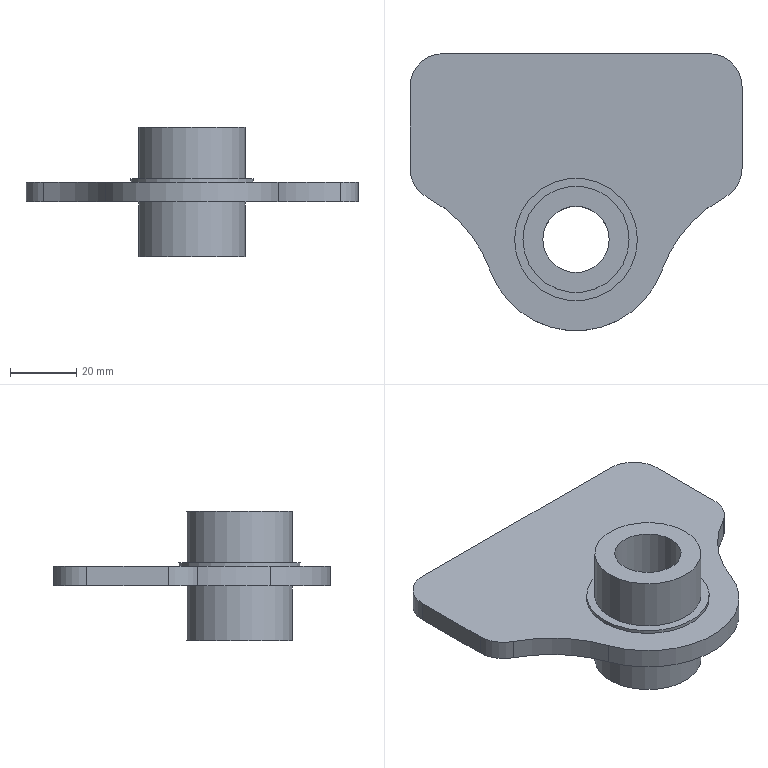Part | NX | 1 solid | 19 faces | box 100 x 83.5 x 39 mm | volume 52937 mm3 | cylinder 11 | plane 8 | commonest cylinder face diameters 20 x5 32 x2 80 x2 37 x1 55 x1
STEP:
#1=CARTESIAN_POINT('',(-18.8,6.519,-22.5));
#2=VERTEX_POINT('',#1);
#3=CARTESIAN_POINT('',(-34.8,6.519,-22.5));
#4=DIRECTION('',(0.,0.,1.));
#5=DIRECTION('',(1.,0.,0.));
#6=AXIS2_PLACEMENT_3D('',#3,#4,#5);
#7=CIRCLE('',#6,16.);
#8=EDGE_CURVE('',#2,#2,#7,.T.);
#9=ORIENTED_EDGE('',*,*,#8,.F.);
#10=EDGE_LOOP('',(#9));
#11=FACE_BOUND('',#10,.T.);
#12=CARTESIAN_POINT('',(-24.8,6.519,-22.5));
#13=VERTEX_POINT('',#12);
#14=CARTESIAN_POINT('',(-34.8,6.519,-22.5));
#15=DIRECTION('',(0.,0.,1.));
#16=DIRECTION('',(1.,0.,0.));
#17=AXIS2_PLACEMENT_3D('',#14,#15,#16);
#18=CIRCLE('',#17,10.);
#19=EDGE_CURVE('',#13,#13,#18,.T.);
#20=ORIENTED_EDGE('',*,*,#19,.T.);
#21=EDGE_LOOP('',(#20));
#22=FACE_BOUND('',#21,.T.);
#23=CARTESIAN_POINT('',(-34.8,6.519,-22.5));
#24=DIRECTION('',(0.,0.,1.));
#25=DIRECTION('',(1.,0.,0.));
#26=AXIS2_PLACEMENT_3D('',#23,#24,#25);
#27=PLANE('',#26);
#28=ADVANCED_FACE('',(#11,#22),#27,.F.);
#29=CARTESIAN_POINT('',(-18.8,6.519,-6.));
#30=VERTEX_POINT('',#29);
#31=CARTESIAN_POINT('',(-34.8,6.519,-6.));
#32=DIRECTION('',(0.,0.,1.));
#33=DIRECTION('',(1.,0.,0.));
#34=AXIS2_PLACEMENT_3D('',#31,#32,#33);
#35=CIRCLE('',#34,16.);
#36=EDGE_CURVE('',#30,#30,#35,.T.);
#37=ORIENTED_EDGE('',*,*,#36,.T.);
#38=EDGE_LOOP('',(#37));
#39=FACE_BOUND('',#38,.T.);
#40=CARTESIAN_POINT('',(-60.71,-2.696,-6.));
#41=VERTEX_POINT('',#40);
#42=CARTESIAN_POINT('',(-8.889,-2.696,-6.));
#43=VERTEX_POINT('',#42);
#44=CARTESIAN_POINT('',(-34.8,6.519,-6.));
#45=DIRECTION('',(0.,0.,1.));
#46=DIRECTION('',(1.,0.,0.));
#47=AXIS2_PLACEMENT_3D('',#44,#45,#46);
#48=CIRCLE('',#47,27.5);
#49=EDGE_CURVE('',#41,#43,#48,.T.);
#50=ORIENTED_EDGE('',*,*,#49,.F.);
#51=CARTESIAN_POINT('',(-79.519,19.166,-6.));
#52=VERTEX_POINT('',#51);
#53=CARTESIAN_POINT('',(-98.397,-16.099,-6.));
#54=DIRECTION('',(0.,0.,-1.));
#55=DIRECTION('',(1.,0.,0.));
#56=AXIS2_PLACEMENT_3D('',#53,#54,#55);
#57=CIRCLE('',#56,40.);
#58=EDGE_CURVE('',#52,#41,#57,.T.);
#59=ORIENTED_EDGE('',*,*,#58,.F.);
#60=CARTESIAN_POINT('',(-84.8,27.982,-6.));
#61=VERTEX_POINT('',#60);
#62=CARTESIAN_POINT('',(-74.8,27.982,-6.));
#63=DIRECTION('',(0.,0.,1.));
#64=DIRECTION('',(1.,0.,0.));
#65=AXIS2_PLACEMENT_3D('',#62,#63,#64);
#66=CIRCLE('',#65,10.);
#67=EDGE_CURVE('',#61,#52,#66,.T.);
#68=ORIENTED_EDGE('',*,*,#67,.F.);
#69=CARTESIAN_POINT('',(-84.8,52.519,-6.));
#70=VERTEX_POINT('',#69);
#71=CARTESIAN_POINT('',(-84.8,52.519,-6.));
#72=DIRECTION('',(0.,-1.,0.));
#73=VECTOR('',#72,1000.);
#74=LINE('',#71,#73);
#75=EDGE_CURVE('',#70,#61,#74,.T.);
#76=ORIENTED_EDGE('',*,*,#75,.F.);
#77=CARTESIAN_POINT('',(-74.8,62.519,-6.));
#78=VERTEX_POINT('',#77);
#79=CARTESIAN_POINT('',(-74.8,52.519,-6.));
#80=DIRECTION('',(0.,0.,1.));
#81=DIRECTION('',(1.,0.,0.));
#82=AXIS2_PLACEMENT_3D('',#79,#80,#81);
#83=CIRCLE('',#82,10.);
#84=EDGE_CURVE('',#78,#70,#83,.T.);
#85=ORIENTED_EDGE('',*,*,#84,.F.);
#86=CARTESIAN_POINT('',(5.2,62.519,-6.));
#87=VERTEX_POINT('',#86);
#88=CARTESIAN_POINT('',(5.2,62.519,-6.));
#89=DIRECTION('',(-1.,0.,0.));
#90=VECTOR('',#89,1000.);
#91=LINE('',#88,#90);
#92=EDGE_CURVE('',#87,#78,#91,.T.);
#93=ORIENTED_EDGE('',*,*,#92,.F.);
#94=CARTESIAN_POINT('',(15.2,52.519,-6.));
#95=VERTEX_POINT('',#94);
#96=CARTESIAN_POINT('',(5.2,52.519,-6.));
#97=DIRECTION('',(0.,0.,1.));
#98=DIRECTION('',(1.,0.,0.));
#99=AXIS2_PLACEMENT_3D('',#96,#97,#98);
#100=CIRCLE('',#99,10.);
#101=EDGE_CURVE('',#95,#87,#100,.T.);
#102=ORIENTED_EDGE('',*,*,#101,.F.);
#103=CARTESIAN_POINT('',(15.2,27.982,-6.));
#104=VERTEX_POINT('',#103);
#105=CARTESIAN_POINT('',(15.2,27.982,-6.));
#106=DIRECTION('',(0.,1.,0.));
#107=VECTOR('',#106,1000.);
#108=LINE('',#105,#107);
#109=EDGE_CURVE('',#104,#95,#108,.T.);
#110=ORIENTED_EDGE('',*,*,#109,.F.);
#111=CARTESIAN_POINT('',(9.92,19.166,-6.));
#112=VERTEX_POINT('',#111);
#113=CARTESIAN_POINT('',(5.2,27.982,-6.));
#114=DIRECTION('',(0.,0.,1.));
#115=DIRECTION('',(1.,0.,0.));
#116=AXIS2_PLACEMENT_3D('',#113,#114,#115);
#117=CIRCLE('',#116,10.);
#118=EDGE_CURVE('',#112,#104,#117,.T.);
#119=ORIENTED_EDGE('',*,*,#118,.F.);
#120=CARTESIAN_POINT('',(28.798,-16.099,-6.));
#121=DIRECTION('',(0.,0.,-1.));
#122=DIRECTION('',(1.,0.,0.));
#123=AXIS2_PLACEMENT_3D('',#120,#121,#122);
#124=CIRCLE('',#123,40.);
#125=EDGE_CURVE('',#43,#112,#124,.T.);
#126=ORIENTED_EDGE('',*,*,#125,.F.);
#127=EDGE_LOOP('',(#50,#59,#68,#76,#85,#93,#102,#110,#119,#126));
#128=FACE_BOUND('',#127,.T.);
#129=CARTESIAN_POINT('',(-34.8,6.519,-6.));
#130=DIRECTION('',(0.,0.,1.));
#131=DIRECTION('',(1.,0.,0.));
#132=AXIS2_PLACEMENT_3D('',#129,#130,#131);
#133=PLANE('',#132);
#134=ADVANCED_FACE('',(#39,#128),#133,.F.);
#135=CARTESIAN_POINT('',(-60.71,-2.696,0.));
#136=VERTEX_POINT('',#135);
#137=CARTESIAN_POINT('',(-8.889,-2.696,0.));
#138=VERTEX_POINT('',#137);
#139=CARTESIAN_POINT('',(-34.8,6.519,0.));
#140=DIRECTION('',(0.,0.,1.));
#141=DIRECTION('',(1.,0.,0.));
#142=AXIS2_PLACEMENT_3D('',#139,#140,#141);
#143=CIRCLE('',#142,27.5);
#144=EDGE_CURVE('',#136,#138,#143,.T.);
#145=ORIENTED_EDGE('',*,*,#144,.F.);
#146=CARTESIAN_POINT('',(-60.71,-2.696,-6.));
#147=DIRECTION('',(0.,0.,1.));
#148=VECTOR('',#147,1000.);
#149=LINE('',#146,#148);
#150=EDGE_CURVE('',#41,#136,#149,.T.);
#151=ORIENTED_EDGE('',*,*,#150,.F.);
#152=ORIENTED_EDGE('',*,*,#49,.T.);
#153=CARTESIAN_POINT('',(-8.889,-2.696,-6.));
#154=DIRECTION('',(0.,0.,1.));
#155=VECTOR('',#154,1000.);
#156=LINE('',#153,#155);
#157=EDGE_CURVE('',#43,#138,#156,.T.);
#158=ORIENTED_EDGE('',*,*,#157,.T.);
#159=EDGE_LOOP('',(#145,#151,#152,#158));
#160=FACE_BOUND('',#159,.T.);
#161=CARTESIAN_POINT('',(-34.8,6.519,-6.));
#162=DIRECTION('',(0.,0.,1.));
#163=DIRECTION('',(1.,0.,0.));
#164=AXIS2_PLACEMENT_3D('',#161,#162,#163);
#165=CYLINDRICAL_SURFACE('',#164,27.5);
#166=ADVANCED_FACE('',(#160),#165,.T.);
#167=CARTESIAN_POINT('',(9.92,19.166,0.));
#168=VERTEX_POINT('',#167);
#169=CARTESIAN_POINT('',(28.798,-16.099,0.));
#170=DIRECTION('',(0.,0.,-1.));
#171=DIRECTION('',(1.,0.,0.));
#172=AXIS2_PLACEMENT_3D('',#169,#170,#171);
#173=CIRCLE('',#172,40.);
#174=EDGE_CURVE('',#138,#168,#173,.T.);
#175=ORIENTED_EDGE('',*,*,#174,.F.);
#176=ORIENTED_EDGE('',*,*,#157,.F.);
#177=ORIENTED_EDGE('',*,*,#125,.T.);
#178=CARTESIAN_POINT('',(9.92,19.166,-6.));
#179=DIRECTION('',(0.,0.,1.));
#180=VECTOR('',#179,1000.);
#181=LINE('',#178,#180);
#182=EDGE_CURVE('',#112,#168,#181,.T.);
#183=ORIENTED_EDGE('',*,*,#182,.T.);
#184=EDGE_LOOP('',(#175,#176,#177,#183));
#185=FACE_BOUND('',#184,.T.);
#186=CARTESIAN_POINT('',(28.798,-16.099,-6.));
#187=DIRECTION('',(0.,0.,1.));
#188=DIRECTION('',(1.,0.,0.));
#189=AXIS2_PLACEMENT_3D('',#186,#187,#188);
#190=CYLINDRICAL_SURFACE('',#189,40.);
#191=ADVANCED_FACE('',(#185),#190,.F.);
#192=CARTESIAN_POINT('',(15.2,27.982,0.));
#193=VERTEX_POINT('',#192);
#194=CARTESIAN_POINT('',(5.2,27.982,0.));
#195=DIRECTION('',(0.,0.,1.));
#196=DIRECTION('',(1.,0.,0.));
#197=AXIS2_PLACEMENT_3D('',#194,#195,#196);
#198=CIRCLE('',#197,10.);
#199=EDGE_CURVE('',#168,#193,#198,.T.);
#200=ORIENTED_EDGE('',*,*,#199,.F.);
#201=ORIENTED_EDGE('',*,*,#182,.F.);
#202=ORIENTED_EDGE('',*,*,#118,.T.);
#203=CARTESIAN_POINT('',(15.2,27.982,-6.));
#204=DIRECTION('',(0.,0.,1.));
#205=VECTOR('',#204,1000.);
#206=LINE('',#203,#205);
#207=EDGE_CURVE('',#104,#193,#206,.T.);
#208=ORIENTED_EDGE('',*,*,#207,.T.);
#209=EDGE_LOOP('',(#200,#201,#202,#208));
#210=FACE_BOUND('',#209,.T.);
#211=CARTESIAN_POINT('',(5.2,27.982,-6.));
#212=DIRECTION('',(0.,0.,1.));
#213=DIRECTION('',(1.,0.,0.));
#214=AXIS2_PLACEMENT_3D('',#211,#212,#213);
#215=CYLINDRICAL_SURFACE('',#214,10.);
#216=ADVANCED_FACE('',(#210),#215,.T.);
#217=CARTESIAN_POINT('',(15.2,52.519,0.));
#218=VERTEX_POINT('',#217);
#219=CARTESIAN_POINT('',(15.2,51.519,0.));
#220=DIRECTION('',(0.,1.,0.));
#221=VECTOR('',#220,1000.);
#222=LINE('',#219,#221);
#223=EDGE_CURVE('',#193,#218,#222,.T.);
#224=ORIENTED_EDGE('',*,*,#223,.F.);
#225=ORIENTED_EDGE('',*,*,#207,.F.);
#226=ORIENTED_EDGE('',*,*,#109,.T.);
#227=CARTESIAN_POINT('',(15.2,52.519,-6.));
#228=DIRECTION('',(0.,0.,1.));
#229=VECTOR('',#228,1000.);
#230=LINE('',#227,#229);
#231=EDGE_CURVE('',#95,#218,#230,.T.);
#232=ORIENTED_EDGE('',*,*,#231,.T.);
#233=EDGE_LOOP('',(#224,#225,#226,#232));
#234=FACE_BOUND('',#233,.T.);
#235=CARTESIAN_POINT('',(15.2,51.519,-6.));
#236=DIRECTION('',(1.,0.,0.));
#237=DIRECTION('',(0.,1.,0.));
#238=AXIS2_PLACEMENT_3D('',#235,#236,#237);
#239=PLANE('',#238);
#240=ADVANCED_FACE('',(#234),#239,.T.);
#241=CARTESIAN_POINT('',(5.2,62.519,0.));
#242=VERTEX_POINT('',#241);
#243=CARTESIAN_POINT('',(5.2,52.519,0.));
#244=DIRECTION('',(0.,0.,1.));
#245=DIRECTION('',(1.,0.,0.));
#246=AXIS2_PLACEMENT_3D('',#243,#244,#245);
#247=CIRCLE('',#246,10.);
#248=EDGE_CURVE('',#218,#242,#247,.T.);
#249=ORIENTED_EDGE('',*,*,#248,.F.);
#250=ORIENTED_EDGE('',*,*,#231,.F.);
#251=ORIENTED_EDGE('',*,*,#101,.T.);
#252=CARTESIAN_POINT('',(5.2,62.519,-6.));
#253=DIRECTION('',(0.,0.,1.));
#254=VECTOR('',#253,1000.);
#255=LINE('',#252,#254);
#256=EDGE_CURVE('',#87,#242,#255,.T.);
#257=ORIENTED_EDGE('',*,*,#256,.T.);
#258=EDGE_LOOP('',(#249,#250,#251,#257));
#259=FACE_BOUND('',#258,.T.);
#260=CARTESIAN_POINT('',(5.2,52.519,-6.));
#261=DIRECTION('',(0.,0.,1.));
#262=DIRECTION('',(1.,0.,0.));
#263=AXIS2_PLACEMENT_3D('',#260,#261,#262);
#264=CYLINDRICAL_SURFACE('',#263,10.);
#265=ADVANCED_FACE('',(#259),#264,.T.);
#266=CARTESIAN_POINT('',(-74.8,62.519,0.));
#267=VERTEX_POINT('',#266);
#268=CARTESIAN_POINT('',(5.2,62.519,0.));
#269=DIRECTION('',(-1.,0.,0.));
#270=VECTOR('',#269,1000.);
#271=LINE('',#268,#270);
#272=EDGE_CURVE('',#242,#267,#271,.T.);
#273=ORIENTED_EDGE('',*,*,#272,.F.);
#274=ORIENTED_EDGE('',*,*,#256,.F.);
#275=ORIENTED_EDGE('',*,*,#92,.T.);
#276=CARTESIAN_POINT('',(-74.8,62.519,-6.));
#277=DIRECTION('',(0.,0.,1.));
#278=VECTOR('',#277,1000.);
#279=LINE('',#276,#278);
#280=EDGE_CURVE('',#78,#267,#279,.T.);
#281=ORIENTED_EDGE('',*,*,#280,.T.);
#282=EDGE_LOOP('',(#273,#274,#275,#281));
#283=FACE_BOUND('',#282,.T.);
#284=CARTESIAN_POINT('',(5.2,62.519,-6.));
#285=DIRECTION('',(0.,1.,0.));
#286=DIRECTION('',(-1.,0.,0.));
#287=AXIS2_PLACEMENT_3D('',#284,#285,#286);
#288=PLANE('',#287);
#289=ADVANCED_FACE('',(#283),#288,.T.);
#290=CARTESIAN_POINT('',(-84.8,52.519,0.));
#291=VERTEX_POINT('',#290);
#292=CARTESIAN_POINT('',(-74.8,52.519,0.));
#293=DIRECTION('',(0.,0.,1.));
#294=DIRECTION('',(1.,0.,0.));
#295=AXIS2_PLACEMENT_3D('',#292,#293,#294);
#296=CIRCLE('',#295,10.);
#297=EDGE_CURVE('',#267,#291,#296,.T.);
#298=ORIENTED_EDGE('',*,*,#297,.F.);
#299=ORIENTED_EDGE('',*,*,#280,.F.);
#300=ORIENTED_EDGE('',*,*,#84,.T.);
#301=CARTESIAN_POINT('',(-84.8,52.519,-6.));
#302=DIRECTION('',(0.,0.,1.));
#303=VECTOR('',#302,1000.);
#304=LINE('',#301,#303);
#305=EDGE_CURVE('',#70,#291,#304,.T.);
#306=ORIENTED_EDGE('',*,*,#305,.T.);
#307=EDGE_LOOP('',(#298,#299,#300,#306));
#308=FACE_BOUND('',#307,.T.);
#309=CARTESIAN_POINT('',(-74.8,52.519,-6.));
#310=DIRECTION('',(0.,0.,1.));
#311=DIRECTION('',(1.,0.,0.));
#312=AXIS2_PLACEMENT_3D('',#309,#310,#311);
#313=CYLINDRICAL_SURFACE('',#312,10.);
#314=ADVANCED_FACE('',(#308),#313,.T.);
#315=CARTESIAN_POINT('',(-84.8,27.982,0.));
#316=VERTEX_POINT('',#315);
#317=CARTESIAN_POINT('',(-84.8,51.519,0.));
#318=DIRECTION('',(0.,-1.,0.));
#319=VECTOR('',#318,1000.);
#320=LINE('',#317,#319);
#321=EDGE_CURVE('',#291,#316,#320,.T.);
#322=ORIENTED_EDGE('',*,*,#321,.F.);
#323=ORIENTED_EDGE('',*,*,#305,.F.);
#324=ORIENTED_EDGE('',*,*,#75,.T.);
#325=CARTESIAN_POINT('',(-84.8,27.982,-6.));
#326=DIRECTION('',(0.,0.,1.));
#327=VECTOR('',#326,1000.);
#328=LINE('',#325,#327);
#329=EDGE_CURVE('',#61,#316,#328,.T.);
#330=ORIENTED_EDGE('',*,*,#329,.T.);
#331=EDGE_LOOP('',(#322,#323,#324,#330));
#332=FACE_BOUND('',#331,.T.);
#333=CARTESIAN_POINT('',(-84.8,51.519,-6.));
#334=DIRECTION('',(-1.,0.,0.));
#335=DIRECTION('',(0.,0.,1.));
#336=AXIS2_PLACEMENT_3D('',#333,#334,#335);
#337=PLANE('',#336);
#338=ADVANCED_FACE('',(#332),#337,.T.);
#339=CARTESIAN_POINT('',(-79.519,19.166,0.));
#340=VERTEX_POINT('',#339);
#341=CARTESIAN_POINT('',(-74.8,27.982,0.));
#342=DIRECTION('',(0.,0.,1.));
#343=DIRECTION('',(1.,0.,0.));
#344=AXIS2_PLACEMENT_3D('',#341,#342,#343);
#345=CIRCLE('',#344,10.);
#346=EDGE_CURVE('',#316,#340,#345,.T.);
#347=ORIENTED_EDGE('',*,*,#346,.F.);
#348=ORIENTED_EDGE('',*,*,#329,.F.);
#349=ORIENTED_EDGE('',*,*,#67,.T.);
#350=CARTESIAN_POINT('',(-79.519,19.166,-6.));
#351=DIRECTION('',(0.,0.,1.));
#352=VECTOR('',#351,1000.);
#353=LINE('',#350,#352);
#354=EDGE_CURVE('',#52,#340,#353,.T.);
#355=ORIENTED_EDGE('',*,*,#354,.T.);
#356=EDGE_LOOP('',(#347,#348,#349,#355));
#357=FACE_BOUND('',#356,.T.);
#358=CARTESIAN_POINT('',(-74.8,27.982,-6.));
#359=DIRECTION('',(0.,0.,1.));
#360=DIRECTION('',(1.,0.,0.));
#361=AXIS2_PLACEMENT_3D('',#358,#359,#360);
#362=CYLINDRICAL_SURFACE('',#361,10.);
#363=ADVANCED_FACE('',(#357),#362,.T.);
#364=CARTESIAN_POINT('',(-98.397,-16.099,0.));
#365=DIRECTION('',(0.,0.,-1.));
#366=DIRECTION('',(1.,0.,0.));
#367=AXIS2_PLACEMENT_3D('',#364,#365,#366);
#368=CIRCLE('',#367,40.);
#369=EDGE_CURVE('',#340,#136,#368,.T.);
#370=ORIENTED_EDGE('',*,*,#369,.F.);
#371=ORIENTED_EDGE('',*,*,#354,.F.);
#372=ORIENTED_EDGE('',*,*,#58,.T.);
#373=ORIENTED_EDGE('',*,*,#150,.T.);
#374=EDGE_LOOP('',(#370,#371,#372,#373));
#375=FACE_BOUND('',#374,.T.);
#376=CARTESIAN_POINT('',(-98.397,-16.099,-6.));
#377=DIRECTION('',(0.,0.,1.));
#378=DIRECTION('',(1.,0.,0.));
#379=AXIS2_PLACEMENT_3D('',#376,#377,#378);
#380=CYLINDRICAL_SURFACE('',#379,40.);
#381=ADVANCED_FACE('',(#375),#380,.F.);
#382=CARTESIAN_POINT('',(-16.3,6.519,0.));
#383=VERTEX_POINT('',#382);
#384=CARTESIAN_POINT('',(-34.8,6.519,0.));
#385=DIRECTION('',(0.,0.,1.));
#386=DIRECTION('',(1.,0.,0.));
#387=AXIS2_PLACEMENT_3D('',#384,#385,#386);
#388=CIRCLE('',#387,18.5);
#389=EDGE_CURVE('',#383,#383,#388,.T.);
#390=ORIENTED_EDGE('',*,*,#389,.F.);
#391=EDGE_LOOP('',(#390));
#392=FACE_BOUND('',#391,.T.);
#393=ORIENTED_EDGE('',*,*,#144,.T.);
#394=ORIENTED_EDGE('',*,*,#174,.T.);
#395=ORIENTED_EDGE('',*,*,#199,.T.);
#396=ORIENTED_EDGE('',*,*,#223,.T.);
#397=ORIENTED_EDGE('',*,*,#248,.T.);
#398=ORIENTED_EDGE('',*,*,#272,.T.);
#399=ORIENTED_EDGE('',*,*,#297,.T.);
#400=ORIENTED_EDGE('',*,*,#321,.T.);
#401=ORIENTED_EDGE('',*,*,#346,.T.);
#402=ORIENTED_EDGE('',*,*,#369,.T.);
#403=EDGE_LOOP('',(#393,#394,#395,#396,#397,#398,#399,#400,#401,#402));
#404=FACE_BOUND('',#403,.T.);
#405=CARTESIAN_POINT('',(-34.8,6.519,0.));
#406=DIRECTION('',(0.,0.,1.));
#407=DIRECTION('',(1.,0.,0.));
#408=AXIS2_PLACEMENT_3D('',#405,#406,#407);
#409=PLANE('',#408);
#410=ADVANCED_FACE('',(#392,#404),#409,.T.);
#411=CARTESIAN_POINT('',(-18.8,6.519,16.5));
#412=VERTEX_POINT('',#411);
#413=CARTESIAN_POINT('',(-34.8,6.519,16.5));
#414=DIRECTION('',(0.,0.,1.));
#415=DIRECTION('',(1.,0.,0.));
#416=AXIS2_PLACEMENT_3D('',#413,#414,#415);
#417=CIRCLE('',#416,16.);
#418=EDGE_CURVE('',#412,#412,#417,.T.);
#419=ORIENTED_EDGE('',*,*,#418,.F.);
#420=EDGE_LOOP('',(#419));
#421=FACE_BOUND('',#420,.T.);
#422=CARTESIAN_POINT('',(-50.8,6.519,1.));
#423=VERTEX_POINT('',#422);
#424=CARTESIAN_POINT('',(-34.8,6.519,1.));
#425=DIRECTION('',(0.,0.,-1.));
#426=DIRECTION('',(-1.,0.,0.));
#427=AXIS2_PLACEMENT_3D('',#424,#425,#426);
#428=CIRCLE('',#427,16.);
#429=EDGE_CURVE('',#423,#423,#428,.T.);
#430=ORIENTED_EDGE('',*,*,#429,.F.);
#431=EDGE_LOOP('',(#430));
#432=FACE_BOUND('',#431,.T.);
#433=CARTESIAN_POINT('',(-34.8,6.519,16.5));
#434=DIRECTION('',(0.,0.,-1.));
#435=DIRECTION('',(-1.,0.,0.));
#436=AXIS2_PLACEMENT_3D('',#433,#434,#435);
#437=CYLINDRICAL_SURFACE('',#436,16.);
#438=ADVANCED_FACE('',(#421,#432),#437,.T.);
#439=ORIENTED_EDGE('',*,*,#19,.F.);
#440=EDGE_LOOP('',(#439));
#441=FACE_BOUND('',#440,.T.);
#442=CARTESIAN_POINT('',(-24.8,6.519,16.5));
#443=VERTEX_POINT('',#442);
#444=CARTESIAN_POINT('',(-34.8,6.519,16.5));
#445=DIRECTION('',(0.,0.,1.));
#446=DIRECTION('',(1.,0.,0.));
#447=AXIS2_PLACEMENT_3D('',#444,#445,#446);
#448=CIRCLE('',#447,10.);
#449=EDGE_CURVE('',#443,#443,#448,.T.);
#450=ORIENTED_EDGE('',*,*,#449,.T.);
#451=EDGE_LOOP('',(#450));
#452=FACE_BOUND('',#451,.T.);
#453=CARTESIAN_POINT('',(-34.8,6.519,16.5));
#454=DIRECTION('',(0.,0.,-1.));
#455=DIRECTION('',(-1.,0.,0.));
#456=AXIS2_PLACEMENT_3D('',#453,#454,#455);
#457=CYLINDRICAL_SURFACE('',#456,10.);
#458=ADVANCED_FACE('',(#441,#452),#457,.F.);
#459=ORIENTED_EDGE('',*,*,#418,.T.);
#460=EDGE_LOOP('',(#459));
#461=FACE_BOUND('',#460,.T.);
#462=ORIENTED_EDGE('',*,*,#449,.F.);
#463=EDGE_LOOP('',(#462));
#464=FACE_BOUND('',#463,.T.);
#465=CARTESIAN_POINT('',(-34.8,6.519,16.5));
#466=DIRECTION('',(0.,0.,1.));
#467=DIRECTION('',(1.,0.,0.));
#468=AXIS2_PLACEMENT_3D('',#465,#466,#467);
#469=PLANE('',#468);
#470=ADVANCED_FACE('',(#461,#464),#469,.T.);
#471=ORIENTED_EDGE('',*,*,#389,.T.);
#472=EDGE_LOOP('',(#471));
#473=FACE_BOUND('',#472,.T.);
#474=CARTESIAN_POINT('',(-16.3,6.519,1.));
#475=VERTEX_POINT('',#474);
#476=CARTESIAN_POINT('',(-34.8,6.519,1.));
#477=DIRECTION('',(0.,0.,-1.));
#478=DIRECTION('',(1.,0.,0.));
#479=AXIS2_PLACEMENT_3D('',#476,#477,#478);
#480=CIRCLE('',#479,18.5);
#481=EDGE_CURVE('',#475,#475,#480,.T.);
#482=ORIENTED_EDGE('',*,*,#481,.T.);
#483=EDGE_LOOP('',(#482));
#484=FACE_BOUND('',#483,.T.);
#485=CARTESIAN_POINT('',(-34.8,6.519,1.));
#486=DIRECTION('',(0.,0.,-1.));
#487=DIRECTION('',(-1.,0.,0.));
#488=AXIS2_PLACEMENT_3D('',#485,#486,#487);
#489=CYLINDRICAL_SURFACE('',#488,18.5);
#490=ADVANCED_FACE('',(#473,#484),#489,.T.);
#491=ORIENTED_EDGE('',*,*,#429,.T.);
#492=EDGE_LOOP('',(#491));
#493=FACE_BOUND('',#492,.T.);
#494=ORIENTED_EDGE('',*,*,#481,.F.);
#495=EDGE_LOOP('',(#494));
#496=FACE_BOUND('',#495,.T.);
#497=CARTESIAN_POINT('',(-34.8,6.519,1.));
#498=DIRECTION('',(0.,0.,-1.));
#499=DIRECTION('',(-1.,0.,0.));
#500=AXIS2_PLACEMENT_3D('',#497,#498,#499);
#501=PLANE('',#500);
#502=ADVANCED_FACE('',(#493,#496),#501,.F.);
#503=ORIENTED_EDGE('',*,*,#8,.T.);
#504=EDGE_LOOP('',(#503));
#505=FACE_BOUND('',#504,.T.);
#506=ORIENTED_EDGE('',*,*,#36,.F.);
#507=EDGE_LOOP('',(#506));
#508=FACE_BOUND('',#507,.T.);
#509=CARTESIAN_POINT('',(-34.8,6.519,-25.));
#510=DIRECTION('',(0.,0.,1.));
#511=DIRECTION('',(1.,0.,0.));
#512=AXIS2_PLACEMENT_3D('',#509,#510,#511);
#513=CYLINDRICAL_SURFACE('',#512,16.);
#514=ADVANCED_FACE('',(#505,#508),#513,.T.);
#515=CLOSED_SHELL('',(#28,#134,#166,#191,#216,#240,#265,#289,#314,#338,#363,#381,#410,#438,#458,#470,#490,#502,#514));
#516=MANIFOLD_SOLID_BREP('',#515);
#517=(LENGTH_UNIT()NAMED_UNIT(*)SI_UNIT(.MILLI.,.METRE.));
#518=UNCERTAINTY_MEASURE_WITH_UNIT(LENGTH_MEASURE(0.00001),#517,'','');
#519=(NAMED_UNIT(*)PLANE_ANGLE_UNIT()SI_UNIT($,.RADIAN.));
#520=(NAMED_UNIT(*)SI_UNIT($,.STERADIAN.)SOLID_ANGLE_UNIT());
#521=(GEOMETRIC_REPRESENTATION_CONTEXT(3)GLOBAL_UNCERTAINTY_ASSIGNED_CONTEXT((#518))GLOBAL_UNIT_ASSIGNED_CONTEXT((#517,#519,#520))REPRESENTATION_CONTEXT('',''));
#522=ADVANCED_BREP_SHAPE_REPRESENTATION('',(#516),#521);